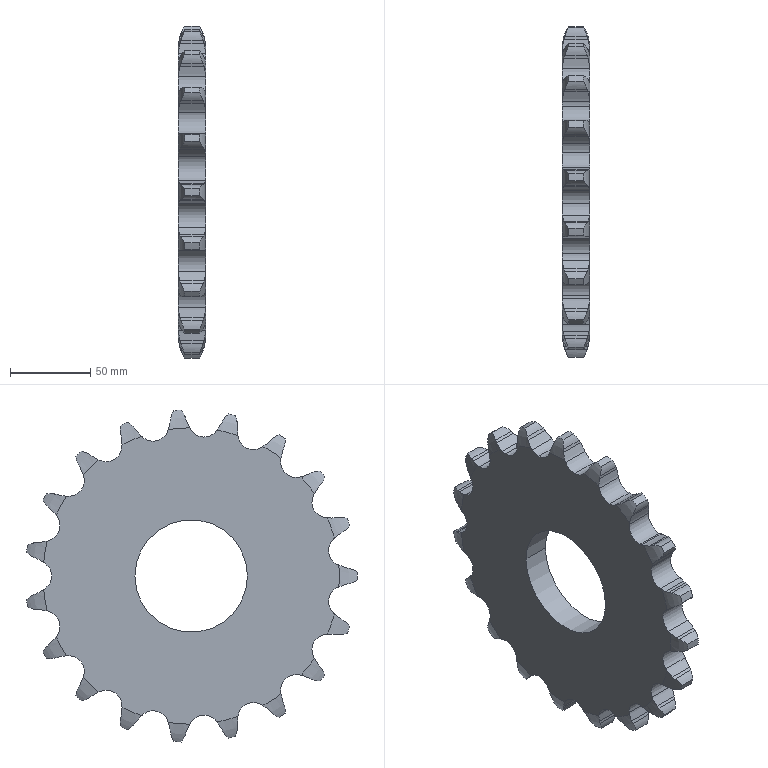Part | STEP file | 果蔬烘干机从动链轮-19齿_20A | 1 solid | 203 faces | box 17 x 205.935 x 206.617 mm | volume 397134 mm3 | cylinder 125 | plane 40 | torus 38 | commonest cylinder face diameters 27.844 x40 49.725 x40 19.245 x24 207 x19 70 x2